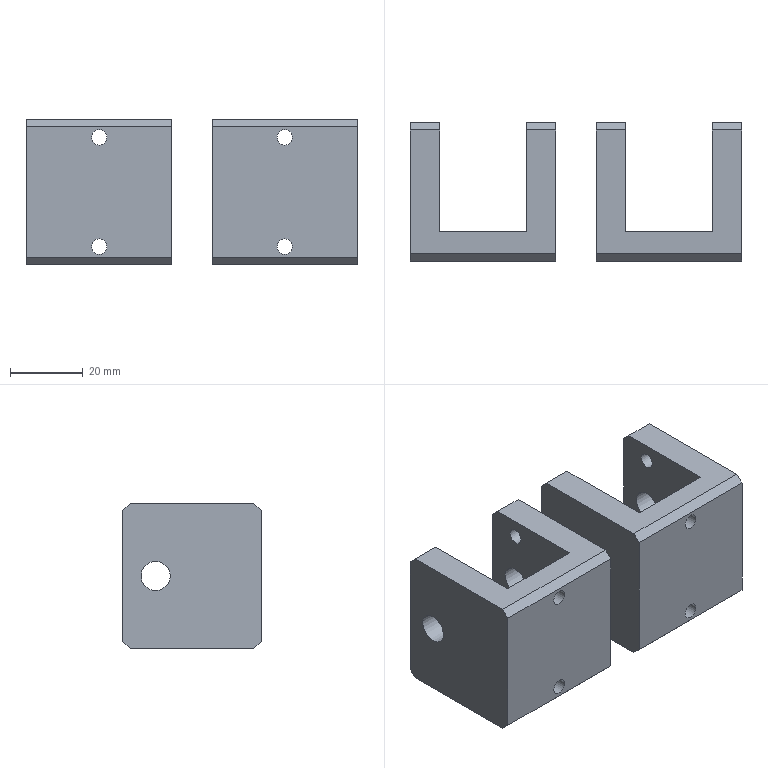Part | 2 solids | 52 faces | box 91 x 38 x 40 mm | volume 60346 mm3 | plane 32 | cylinder 16 | cone 4 | commonest cylinder face diameters 4.2 x12 8 x4
STEP:
#1=CARTESIAN_POINT('',(31.,36.,20.));
#2=VERTEX_POINT('',#1);
#3=CARTESIAN_POINT('',(31.,38.,18.));
#4=VERTEX_POINT('',#3);
#5=CARTESIAN_POINT('',(31.,38.,18.));
#6=DIRECTION('',(0.,0.7071,-0.7071));
#7=VECTOR('',#6,1000.);
#8=LINE('',#5,#7);
#9=EDGE_CURVE('',#2,#4,#8,.T.);
#10=ORIENTED_EDGE('',*,*,#9,.F.);
#11=CARTESIAN_POINT('',(39.,36.,20.));
#12=VERTEX_POINT('',#11);
#13=CARTESIAN_POINT('',(31.,36.,20.));
#14=DIRECTION('',(-1.,0.,0.));
#15=VECTOR('',#14,1000.);
#16=LINE('',#13,#15);
#17=EDGE_CURVE('',#12,#2,#16,.T.);
#18=ORIENTED_EDGE('',*,*,#17,.F.);
#19=CARTESIAN_POINT('',(39.,38.,18.));
#20=VERTEX_POINT('',#19);
#21=CARTESIAN_POINT('',(39.,38.,18.));
#22=DIRECTION('',(0.,-0.7071,0.7071));
#23=VECTOR('',#22,1000.);
#24=LINE('',#21,#23);
#25=EDGE_CURVE('',#20,#12,#24,.T.);
#26=ORIENTED_EDGE('',*,*,#25,.F.);
#27=CARTESIAN_POINT('',(39.,38.,18.));
#28=DIRECTION('',(1.,0.,0.));
#29=VECTOR('',#28,1000.);
#30=LINE('',#27,#29);
#31=EDGE_CURVE('',#4,#20,#30,.T.);
#32=ORIENTED_EDGE('',*,*,#31,.F.);
#33=EDGE_LOOP('',(#10,#18,#26,#32));
#34=FACE_BOUND('',#33,.T.);
#35=CARTESIAN_POINT('',(51.,38.,18.));
#36=DIRECTION('',(0.,0.7071,0.7071));
#37=DIRECTION('',(-1.,0.,0.));
#38=AXIS2_PLACEMENT_3D('',#35,#36,#37);
#39=PLANE('',#38);
#40=ADVANCED_FACE('',(#34),#39,.T.);
#41=CARTESIAN_POINT('',(39.,36.,-20.));
#42=VERTEX_POINT('',#41);
#43=CARTESIAN_POINT('',(39.,38.,-18.));
#44=VERTEX_POINT('',#43);
#45=CARTESIAN_POINT('',(39.,38.,-18.));
#46=DIRECTION('',(0.,0.7071,0.7071));
#47=VECTOR('',#46,1000.);
#48=LINE('',#45,#47);
#49=EDGE_CURVE('',#42,#44,#48,.T.);
#50=ORIENTED_EDGE('',*,*,#49,.F.);
#51=CARTESIAN_POINT('',(31.,36.,-20.));
#52=VERTEX_POINT('',#51);
#53=CARTESIAN_POINT('',(39.,36.,-20.));
#54=DIRECTION('',(1.,0.,0.));
#55=VECTOR('',#54,1000.);
#56=LINE('',#53,#55);
#57=EDGE_CURVE('',#52,#42,#56,.T.);
#58=ORIENTED_EDGE('',*,*,#57,.F.);
#59=CARTESIAN_POINT('',(31.,38.,-18.));
#60=VERTEX_POINT('',#59);
#61=CARTESIAN_POINT('',(31.,38.,-18.));
#62=DIRECTION('',(0.,-0.7071,-0.7071));
#63=VECTOR('',#62,1000.);
#64=LINE('',#61,#63);
#65=EDGE_CURVE('',#60,#52,#64,.T.);
#66=ORIENTED_EDGE('',*,*,#65,.F.);
#67=CARTESIAN_POINT('',(31.,38.,-18.));
#68=DIRECTION('',(-1.,0.,0.));
#69=VECTOR('',#68,1000.);
#70=LINE('',#67,#69);
#71=EDGE_CURVE('',#44,#60,#70,.T.);
#72=ORIENTED_EDGE('',*,*,#71,.F.);
#73=EDGE_LOOP('',(#50,#58,#66,#72));
#74=FACE_BOUND('',#73,.T.);
#75=CARTESIAN_POINT('',(51.,38.,-18.));
#76=DIRECTION('',(0.,0.7071,-0.7071));
#77=DIRECTION('',(1.,0.,0.));
#78=AXIS2_PLACEMENT_3D('',#75,#76,#77);
#79=PLANE('',#78);
#80=ADVANCED_FACE('',(#74),#79,.T.);
#81=CARTESIAN_POINT('',(71.,36.,-20.));
#82=VERTEX_POINT('',#81);
#83=CARTESIAN_POINT('',(71.,38.,-18.));
#84=VERTEX_POINT('',#83);
#85=CARTESIAN_POINT('',(71.,38.,-18.));
#86=DIRECTION('',(0.,0.7071,0.7071));
#87=VECTOR('',#86,1000.);
#88=LINE('',#85,#87);
#89=EDGE_CURVE('',#82,#84,#88,.T.);
#90=ORIENTED_EDGE('',*,*,#89,.F.);
#91=CARTESIAN_POINT('',(63.,36.,-20.));
#92=VERTEX_POINT('',#91);
#93=CARTESIAN_POINT('',(71.,36.,-20.));
#94=DIRECTION('',(1.,0.,0.));
#95=VECTOR('',#94,1000.);
#96=LINE('',#93,#95);
#97=EDGE_CURVE('',#92,#82,#96,.T.);
#98=ORIENTED_EDGE('',*,*,#97,.F.);
#99=CARTESIAN_POINT('',(63.,38.,-18.));
#100=VERTEX_POINT('',#99);
#101=CARTESIAN_POINT('',(63.,38.,-18.));
#102=DIRECTION('',(0.,-0.7071,-0.7071));
#103=VECTOR('',#102,1000.);
#104=LINE('',#101,#103);
#105=EDGE_CURVE('',#100,#92,#104,.T.);
#106=ORIENTED_EDGE('',*,*,#105,.F.);
#107=CARTESIAN_POINT('',(63.,38.,-18.));
#108=DIRECTION('',(-1.,0.,0.));
#109=VECTOR('',#108,1000.);
#110=LINE('',#107,#109);
#111=EDGE_CURVE('',#84,#100,#110,.T.);
#112=ORIENTED_EDGE('',*,*,#111,.F.);
#113=EDGE_LOOP('',(#90,#98,#106,#112));
#114=FACE_BOUND('',#113,.T.);
#115=CARTESIAN_POINT('',(51.,38.,-18.));
#116=DIRECTION('',(0.,0.7071,-0.7071));
#117=DIRECTION('',(1.,0.,0.));
#118=AXIS2_PLACEMENT_3D('',#115,#116,#117);
#119=PLANE('',#118);
#120=ADVANCED_FACE('',(#114),#119,.T.);
#121=CARTESIAN_POINT('',(63.,36.,20.));
#122=VERTEX_POINT('',#121);
#123=CARTESIAN_POINT('',(63.,38.,18.));
#124=VERTEX_POINT('',#123);
#125=CARTESIAN_POINT('',(63.,38.,18.));
#126=DIRECTION('',(0.,0.7071,-0.7071));
#127=VECTOR('',#126,1000.);
#128=LINE('',#125,#127);
#129=EDGE_CURVE('',#122,#124,#128,.T.);
#130=ORIENTED_EDGE('',*,*,#129,.F.);
#131=CARTESIAN_POINT('',(71.,36.,20.));
#132=VERTEX_POINT('',#131);
#133=CARTESIAN_POINT('',(63.,36.,20.));
#134=DIRECTION('',(-1.,0.,0.));
#135=VECTOR('',#134,1000.);
#136=LINE('',#133,#135);
#137=EDGE_CURVE('',#132,#122,#136,.T.);
#138=ORIENTED_EDGE('',*,*,#137,.F.);
#139=CARTESIAN_POINT('',(71.,38.,18.));
#140=VERTEX_POINT('',#139);
#141=CARTESIAN_POINT('',(71.,38.,18.));
#142=DIRECTION('',(0.,-0.7071,0.7071));
#143=VECTOR('',#142,1000.);
#144=LINE('',#141,#143);
#145=EDGE_CURVE('',#140,#132,#144,.T.);
#146=ORIENTED_EDGE('',*,*,#145,.F.);
#147=CARTESIAN_POINT('',(71.,38.,18.));
#148=DIRECTION('',(1.,0.,0.));
#149=VECTOR('',#148,1000.);
#150=LINE('',#147,#149);
#151=EDGE_CURVE('',#124,#140,#150,.T.);
#152=ORIENTED_EDGE('',*,*,#151,.F.);
#153=EDGE_LOOP('',(#130,#138,#146,#152));
#154=FACE_BOUND('',#153,.T.);
#155=CARTESIAN_POINT('',(51.,38.,18.));
#156=DIRECTION('',(0.,0.7071,0.7071));
#157=DIRECTION('',(-1.,0.,0.));
#158=AXIS2_PLACEMENT_3D('',#155,#156,#157);
#159=PLANE('',#158);
#160=ADVANCED_FACE('',(#154),#159,.T.);
#161=CARTESIAN_POINT('',(31.,0.,18.));
#162=VERTEX_POINT('',#161);
#163=CARTESIAN_POINT('',(31.,2.,20.));
#164=VERTEX_POINT('',#163);
#165=CARTESIAN_POINT('',(31.,2.,20.));
#166=DIRECTION('',(0.,0.7071,0.7071));
#167=VECTOR('',#166,1000.);
#168=LINE('',#165,#167);
#169=EDGE_CURVE('',#162,#164,#168,.T.);
#170=ORIENTED_EDGE('',*,*,#169,.F.);
#171=CARTESIAN_POINT('',(71.,0.,18.));
#172=VERTEX_POINT('',#171);
#173=CARTESIAN_POINT('',(51.,0.,18.));
#174=DIRECTION('',(-1.,0.,0.));
#175=VECTOR('',#174,1000.);
#176=LINE('',#173,#175);
#177=EDGE_CURVE('',#172,#162,#176,.T.);
#178=ORIENTED_EDGE('',*,*,#177,.F.);
#179=CARTESIAN_POINT('',(71.,2.,20.));
#180=VERTEX_POINT('',#179);
#181=CARTESIAN_POINT('',(71.,2.,20.));
#182=DIRECTION('',(0.,-0.7071,-0.7071));
#183=VECTOR('',#182,1000.);
#184=LINE('',#181,#183);
#185=EDGE_CURVE('',#180,#172,#184,.T.);
#186=ORIENTED_EDGE('',*,*,#185,.F.);
#187=CARTESIAN_POINT('',(31.,2.,20.));
#188=DIRECTION('',(1.,0.,0.));
#189=VECTOR('',#188,1000.);
#190=LINE('',#187,#189);
#191=EDGE_CURVE('',#164,#180,#190,.T.);
#192=ORIENTED_EDGE('',*,*,#191,.F.);
#193=EDGE_LOOP('',(#170,#178,#186,#192));
#194=FACE_BOUND('',#193,.T.);
#195=CARTESIAN_POINT('',(31.,2.,20.));
#196=DIRECTION('',(0.,0.7071,-0.7071));
#197=DIRECTION('',(1.,0.,0.));
#198=AXIS2_PLACEMENT_3D('',#195,#196,#197);
#199=PLANE('',#198);
#200=ADVANCED_FACE('',(#194),#199,.F.);
#201=CARTESIAN_POINT('',(71.,0.,-18.));
#202=VERTEX_POINT('',#201);
#203=CARTESIAN_POINT('',(71.,2.,-20.));
#204=VERTEX_POINT('',#203);
#205=CARTESIAN_POINT('',(71.,2.,-20.));
#206=DIRECTION('',(0.,0.7071,-0.7071));
#207=VECTOR('',#206,1000.);
#208=LINE('',#205,#207);
#209=EDGE_CURVE('',#202,#204,#208,.T.);
#210=ORIENTED_EDGE('',*,*,#209,.F.);
#211=CARTESIAN_POINT('',(31.,0.,-18.));
#212=VERTEX_POINT('',#211);
#213=CARTESIAN_POINT('',(51.,0.,-18.));
#214=DIRECTION('',(1.,0.,0.));
#215=VECTOR('',#214,1000.);
#216=LINE('',#213,#215);
#217=EDGE_CURVE('',#212,#202,#216,.T.);
#218=ORIENTED_EDGE('',*,*,#217,.F.);
#219=CARTESIAN_POINT('',(31.,2.,-20.));
#220=VERTEX_POINT('',#219);
#221=CARTESIAN_POINT('',(31.,2.,-20.));
#222=DIRECTION('',(0.,-0.7071,0.7071));
#223=VECTOR('',#222,1000.);
#224=LINE('',#221,#223);
#225=EDGE_CURVE('',#220,#212,#224,.T.);
#226=ORIENTED_EDGE('',*,*,#225,.F.);
#227=CARTESIAN_POINT('',(31.,2.,-20.));
#228=DIRECTION('',(-1.,0.,0.));
#229=VECTOR('',#228,1000.);
#230=LINE('',#227,#229);
#231=EDGE_CURVE('',#204,#220,#230,.T.);
#232=ORIENTED_EDGE('',*,*,#231,.F.);
#233=EDGE_LOOP('',(#210,#218,#226,#232));
#234=FACE_BOUND('',#233,.T.);
#235=CARTESIAN_POINT('',(31.,2.,-20.));
#236=DIRECTION('',(0.,0.7071,0.7071));
#237=DIRECTION('',(-1.,0.,0.));
#238=AXIS2_PLACEMENT_3D('',#235,#236,#237);
#239=PLANE('',#238);
#240=ADVANCED_FACE('',(#234),#239,.F.);
#241=CARTESIAN_POINT('',(63.,8.,20.));
#242=VERTEX_POINT('',#241);
#243=CARTESIAN_POINT('',(63.,8.,-20.));
#244=VERTEX_POINT('',#243);
#245=CARTESIAN_POINT('',(63.,8.,20.));
#246=DIRECTION('',(0.,0.,-1.));
#247=VECTOR('',#246,1000.);
#248=LINE('',#245,#247);
#249=EDGE_CURVE('',#242,#244,#248,.T.);
#250=ORIENTED_EDGE('',*,*,#249,.T.);
#251=CARTESIAN_POINT('',(39.,8.,-20.));
#252=VERTEX_POINT('',#251);
#253=CARTESIAN_POINT('',(39.,8.,-20.));
#254=DIRECTION('',(-1.,0.,0.));
#255=VECTOR('',#254,1000.);
#256=LINE('',#253,#255);
#257=EDGE_CURVE('',#244,#252,#256,.T.);
#258=ORIENTED_EDGE('',*,*,#257,.T.);
#259=CARTESIAN_POINT('',(39.,8.,20.));
#260=VERTEX_POINT('',#259);
#261=CARTESIAN_POINT('',(39.,8.,20.));
#262=DIRECTION('',(0.,0.,1.));
#263=VECTOR('',#262,1000.);
#264=LINE('',#261,#263);
#265=EDGE_CURVE('',#252,#260,#264,.T.);
#266=ORIENTED_EDGE('',*,*,#265,.T.);
#267=CARTESIAN_POINT('',(39.,8.,20.));
#268=DIRECTION('',(1.,0.,0.));
#269=VECTOR('',#268,1000.);
#270=LINE('',#267,#269);
#271=EDGE_CURVE('',#260,#242,#270,.T.);
#272=ORIENTED_EDGE('',*,*,#271,.T.);
#273=EDGE_LOOP('',(#250,#258,#266,#272));
#274=FACE_BOUND('',#273,.T.);
#275=CARTESIAN_POINT('',(51.,8.,-17.1));
#276=VERTEX_POINT('',#275);
#277=CARTESIAN_POINT('',(51.,8.,-15.));
#278=DIRECTION('',(0.,-1.,0.));
#279=DIRECTION('',(0.,0.,-1.));
#280=AXIS2_PLACEMENT_3D('',#277,#278,#279);
#281=CIRCLE('',#280,2.1);
#282=EDGE_CURVE('',#276,#276,#281,.T.);
#283=ORIENTED_EDGE('',*,*,#282,.T.);
#284=EDGE_LOOP('',(#283));
#285=FACE_BOUND('',#284,.T.);
#286=CARTESIAN_POINT('',(51.,8.,12.9));
#287=VERTEX_POINT('',#286);
#288=CARTESIAN_POINT('',(51.,8.,15.));
#289=DIRECTION('',(0.,-1.,0.));
#290=DIRECTION('',(0.,0.,-1.));
#291=AXIS2_PLACEMENT_3D('',#288,#289,#290);
#292=CIRCLE('',#291,2.1);
#293=EDGE_CURVE('',#287,#287,#292,.T.);
#294=ORIENTED_EDGE('',*,*,#293,.T.);
#295=EDGE_LOOP('',(#294));
#296=FACE_BOUND('',#295,.T.);
#297=CARTESIAN_POINT('',(51.,8.,0.));
#298=DIRECTION('',(0.,-1.,0.));
#299=DIRECTION('',(0.,0.,-1.));
#300=AXIS2_PLACEMENT_3D('',#297,#298,#299);
#301=PLANE('',#300);
#302=ADVANCED_FACE('',(#274,#285,#296),#301,.F.);
#303=CARTESIAN_POINT('',(39.,8.,-20.));
#304=DIRECTION('',(0.,1.,0.));
#305=VECTOR('',#304,1000.);
#306=LINE('',#303,#305);
#307=EDGE_CURVE('',#252,#42,#306,.T.);
#308=ORIENTED_EDGE('',*,*,#307,.T.);
#309=ORIENTED_EDGE('',*,*,#49,.T.);
#310=CARTESIAN_POINT('',(39.,38.,20.));
#311=DIRECTION('',(0.,0.,1.));
#312=VECTOR('',#311,1000.);
#313=LINE('',#310,#312);
#314=EDGE_CURVE('',#44,#20,#313,.T.);
#315=ORIENTED_EDGE('',*,*,#314,.T.);
#316=ORIENTED_EDGE('',*,*,#25,.T.);
#317=CARTESIAN_POINT('',(39.,8.,20.));
#318=DIRECTION('',(0.,1.,0.));
#319=VECTOR('',#318,1000.);
#320=LINE('',#317,#319);
#321=EDGE_CURVE('',#260,#12,#320,.T.);
#322=ORIENTED_EDGE('',*,*,#321,.F.);
#323=ORIENTED_EDGE('',*,*,#265,.F.);
#324=EDGE_LOOP('',(#308,#309,#315,#316,#322,#323));
#325=FACE_BOUND('',#324,.T.);
#326=CARTESIAN_POINT('',(39.,29.,4.));
#327=VERTEX_POINT('',#326);
#328=CARTESIAN_POINT('',(39.,29.,0.));
#329=DIRECTION('',(-1.,0.,0.));
#330=DIRECTION('',(0.,0.,1.));
#331=AXIS2_PLACEMENT_3D('',#328,#329,#330);
#332=CIRCLE('',#331,4.);
#333=EDGE_CURVE('',#327,#327,#332,.T.);
#334=ORIENTED_EDGE('',*,*,#333,.T.);
#335=EDGE_LOOP('',(#334));
#336=FACE_BOUND('',#335,.T.);
#337=CARTESIAN_POINT('',(39.,8.,20.));
#338=DIRECTION('',(-1.,0.,0.));
#339=DIRECTION('',(0.,0.,1.));
#340=AXIS2_PLACEMENT_3D('',#337,#338,#339);
#341=PLANE('',#340);
#342=ADVANCED_FACE('',(#325,#336),#341,.F.);
#343=CARTESIAN_POINT('',(63.,8.,20.));
#344=DIRECTION('',(0.,1.,0.));
#345=VECTOR('',#344,1000.);
#346=LINE('',#343,#345);
#347=EDGE_CURVE('',#242,#122,#346,.T.);
#348=ORIENTED_EDGE('',*,*,#347,.T.);
#349=ORIENTED_EDGE('',*,*,#129,.T.);
#350=CARTESIAN_POINT('',(63.,38.,20.));
#351=DIRECTION('',(0.,0.,-1.));
#352=VECTOR('',#351,1000.);
#353=LINE('',#350,#352);
#354=EDGE_CURVE('',#124,#100,#353,.T.);
#355=ORIENTED_EDGE('',*,*,#354,.T.);
#356=ORIENTED_EDGE('',*,*,#105,.T.);
#357=CARTESIAN_POINT('',(63.,8.,-20.));
#358=DIRECTION('',(0.,1.,0.));
#359=VECTOR('',#358,1000.);
#360=LINE('',#357,#359);
#361=EDGE_CURVE('',#244,#92,#360,.T.);
#362=ORIENTED_EDGE('',*,*,#361,.F.);
#363=ORIENTED_EDGE('',*,*,#249,.F.);
#364=EDGE_LOOP('',(#348,#349,#355,#356,#362,#363));
#365=FACE_BOUND('',#364,.T.);
#366=CARTESIAN_POINT('',(63.,29.,-4.));
#367=VERTEX_POINT('',#366);
#368=CARTESIAN_POINT('',(63.,29.,0.));
#369=DIRECTION('',(1.,0.,0.));
#370=DIRECTION('',(0.,0.,-1.));
#371=AXIS2_PLACEMENT_3D('',#368,#369,#370);
#372=CIRCLE('',#371,4.);
#373=EDGE_CURVE('',#367,#367,#372,.T.);
#374=ORIENTED_EDGE('',*,*,#373,.T.);
#375=EDGE_LOOP('',(#374));
#376=FACE_BOUND('',#375,.T.);
#377=CARTESIAN_POINT('',(63.,29.,12.9));
#378=VERTEX_POINT('',#377);
#379=CARTESIAN_POINT('',(63.,29.,15.));
#380=DIRECTION('',(1.,0.,0.));
#381=DIRECTION('',(0.,0.,-1.));
#382=AXIS2_PLACEMENT_3D('',#379,#380,#381);
#383=CIRCLE('',#382,2.1);
#384=EDGE_CURVE('',#378,#378,#383,.T.);
#385=ORIENTED_EDGE('',*,*,#384,.T.);
#386=EDGE_LOOP('',(#385));
#387=FACE_BOUND('',#386,.T.);
#388=CARTESIAN_POINT('',(63.,29.,-17.1));
#389=VERTEX_POINT('',#388);
#390=CARTESIAN_POINT('',(63.,29.,-15.));
#391=DIRECTION('',(1.,0.,0.));
#392=DIRECTION('',(0.,0.,-1.));
#393=AXIS2_PLACEMENT_3D('',#390,#391,#392);
#394=CIRCLE('',#393,2.1);
#395=EDGE_CURVE('',#389,#389,#394,.T.);
#396=ORIENTED_EDGE('',*,*,#395,.T.);
#397=EDGE_LOOP('',(#396));
#398=FACE_BOUND('',#397,.T.);
#399=CARTESIAN_POINT('',(63.,8.,20.));
#400=DIRECTION('',(1.,0.,0.));
#401=DIRECTION('',(0.,0.,-1.));
#402=AXIS2_PLACEMENT_3D('',#399,#400,#401);
#403=PLANE('',#402);
#404=ADVANCED_FACE('',(#365,#376,#387,#398),#403,.F.);
#405=CARTESIAN_POINT('',(31.,0.,-20.));
#406=DIRECTION('',(0.,0.,1.));
#407=VECTOR('',#406,1000.);
#408=LINE('',#405,#407);
#409=EDGE_CURVE('',#212,#162,#408,.T.);
#410=ORIENTED_EDGE('',*,*,#409,.F.);
#411=ORIENTED_EDGE('',*,*,#217,.T.);
#412=CARTESIAN_POINT('',(71.,0.,-20.));
#413=DIRECTION('',(0.,0.,-1.));
#414=VECTOR('',#413,1000.);
#415=LINE('',#412,#414);
#416=EDGE_CURVE('',#172,#202,#415,.T.);
#417=ORIENTED_EDGE('',*,*,#416,.F.);
#418=ORIENTED_EDGE('',*,*,#177,.T.);
#419=EDGE_LOOP('',(#410,#411,#417,#418));
#420=FACE_BOUND('',#419,.T.);
#421=CARTESIAN_POINT('',(51.,0.,-17.1));
#422=VERTEX_POINT('',#421);
#423=CARTESIAN_POINT('',(51.,0.,-15.));
#424=DIRECTION('',(0.,-1.,0.));
#425=DIRECTION('',(0.,0.,-1.));
#426=AXIS2_PLACEMENT_3D('',#423,#424,#425);
#427=CIRCLE('',#426,2.1);
#428=EDGE_CURVE('',#422,#422,#427,.T.);
#429=ORIENTED_EDGE('',*,*,#428,.F.);
#430=EDGE_LOOP('',(#429));
#431=FACE_BOUND('',#430,.T.);
#432=CARTESIAN_POINT('',(51.,0.,12.9));
#433=VERTEX_POINT('',#432);
#434=CARTESIAN_POINT('',(51.,0.,15.));
#435=DIRECTION('',(0.,-1.,0.));
#436=DIRECTION('',(0.,0.,-1.));
#437=AXIS2_PLACEMENT_3D('',#434,#435,#436);
#438=CIRCLE('',#437,2.1);
#439=EDGE_CURVE('',#433,#433,#438,.T.);
#440=ORIENTED_EDGE('',*,*,#439,.F.);
#441=EDGE_LOOP('',(#440));
#442=FACE_BOUND('',#441,.T.);
#443=CARTESIAN_POINT('',(51.,0.,0.));
#444=DIRECTION('',(0.,1.,0.));
#445=DIRECTION('',(0.,0.,1.));
#446=AXIS2_PLACEMENT_3D('',#443,#444,#445);
#447=PLANE('',#446);
#448=ADVANCED_FACE('',(#420,#431,#442),#447,.F.);
#449=ORIENTED_EDGE('',*,*,#314,.F.);
#450=ORIENTED_EDGE('',*,*,#71,.T.);
#451=CARTESIAN_POINT('',(31.,38.,-20.));
#452=DIRECTION('',(0.,0.,1.));
#453=VECTOR('',#452,1000.);
#454=LINE('',#451,#453);
#455=EDGE_CURVE('',#60,#4,#454,.T.);
#456=ORIENTED_EDGE('',*,*,#455,.T.);
#457=ORIENTED_EDGE('',*,*,#31,.T.);
#458=EDGE_LOOP('',(#449,#450,#456,#457));
#459=FACE_BOUND('',#458,.T.);
#460=CARTESIAN_POINT('',(51.,38.,0.));
#461=DIRECTION('',(0.,1.,0.));
#462=DIRECTION('',(0.,0.,1.));
#463=AXIS2_PLACEMENT_3D('',#460,#461,#462);
#464=PLANE('',#463);
#465=ADVANCED_FACE('',(#459),#464,.T.);
#466=CARTESIAN_POINT('',(31.,38.,20.));
#467=DIRECTION('',(0.,-1.,0.));
#468=VECTOR('',#467,1000.);
#469=LINE('',#466,#468);
#470=EDGE_CURVE('',#2,#164,#469,.T.);
#471=ORIENTED_EDGE('',*,*,#470,.T.);
#472=ORIENTED_EDGE('',*,*,#191,.T.);
#473=CARTESIAN_POINT('',(71.,38.,20.));
#474=DIRECTION('',(0.,-1.,0.));
#475=VECTOR('',#474,1000.);
#476=LINE('',#473,#475);
#477=EDGE_CURVE('',#132,#180,#476,.T.);
#478=ORIENTED_EDGE('',*,*,#477,.F.);
#479=ORIENTED_EDGE('',*,*,#137,.T.);
#480=ORIENTED_EDGE('',*,*,#347,.F.);
#481=ORIENTED_EDGE('',*,*,#271,.F.);
#482=ORIENTED_EDGE('',*,*,#321,.T.);
#483=ORIENTED_EDGE('',*,*,#17,.T.);
#484=EDGE_LOOP('',(#471,#472,#478,#479,#480,#481,#482,#483));
#485=FACE_BOUND('',#484,.T.);
#486=CARTESIAN_POINT('',(31.,38.,20.));
#487=DIRECTION('',(0.,0.,-1.));
#488=DIRECTION('',(-1.,0.,0.));
#489=AXIS2_PLACEMENT_3D('',#486,#487,#488);
#490=PLANE('',#489);
#491=ADVANCED_FACE('',(#485),#490,.F.);
#492=CARTESIAN_POINT('',(31.,38.,-20.));
#493=DIRECTION('',(0.,-1.,0.));
#494=VECTOR('',#493,1000.);
#495=LINE('',#492,#494);
#496=EDGE_CURVE('',#52,#220,#495,.T.);
#497=ORIENTED_EDGE('',*,*,#496,.T.);
#498=ORIENTED_EDGE('',*,*,#225,.T.);
#499=ORIENTED_EDGE('',*,*,#409,.T.);
#500=ORIENTED_EDGE('',*,*,#169,.T.);
#501=ORIENTED_EDGE('',*,*,#470,.F.);
#502=ORIENTED_EDGE('',*,*,#9,.T.);
#503=ORIENTED_EDGE('',*,*,#455,.F.);
#504=ORIENTED_EDGE('',*,*,#65,.T.);
#505=EDGE_LOOP('',(#497,#498,#499,#500,#501,#502,#503,#504));
#506=FACE_BOUND('',#505,.T.);
#507=CARTESIAN_POINT('',(31.,29.,-4.));
#508=VERTEX_POINT('',#507);
#509=CARTESIAN_POINT('',(31.,29.,0.));
#510=DIRECTION('',(1.,0.,0.));
#511=DIRECTION('',(0.,0.,-1.));
#512=AXIS2_PLACEMENT_3D('',#509,#510,#511);
#513=CIRCLE('',#512,4.);
#514=EDGE_CURVE('',#508,#508,#513,.T.);
#515=ORIENTED_EDGE('',*,*,#514,.T.);
#516=EDGE_LOOP('',(#515));
#517=FACE_BOUND('',#516,.T.);
#518=CARTESIAN_POINT('',(31.,38.,-20.));
#519=DIRECTION('',(1.,0.,0.));
#520=DIRECTION('',(0.,0.,-1.));
#521=AXIS2_PLACEMENT_3D('',#518,#519,#520);
#522=PLANE('',#521);
#523=ADVANCED_FACE('',(#506,#517),#522,.F.);
#524=CARTESIAN_POINT('',(71.,38.,-20.));
#525=DIRECTION('',(0.,-1.,0.));
#526=VECTOR('',#525,1000.);
#527=LINE('',#524,#526);
#528=EDGE_CURVE('',#82,#204,#527,.T.);
#529=ORIENTED_EDGE('',*,*,#528,.T.);
#530=ORIENTED_EDGE('',*,*,#231,.T.);
#531=ORIENTED_EDGE('',*,*,#496,.F.);
#532=ORIENTED_EDGE('',*,*,#57,.T.);
#533=ORIENTED_EDGE('',*,*,#307,.F.);
#534=ORIENTED_EDGE('',*,*,#257,.F.);
#535=ORIENTED_EDGE('',*,*,#361,.T.);
#536=ORIENTED_EDGE('',*,*,#97,.T.);
#537=EDGE_LOOP('',(#529,#530,#531,#532,#533,#534,#535,#536));
#538=FACE_BOUND('',#537,.T.);
#539=CARTESIAN_POINT('',(31.,38.,-20.));
#540=DIRECTION('',(0.,0.,1.));
#541=DIRECTION('',(1.,0.,0.));
#542=AXIS2_PLACEMENT_3D('',#539,#540,#541);
#543=PLANE('',#542);
#544=ADVANCED_FACE('',(#538),#543,.F.);
#545=ORIENTED_EDGE('',*,*,#416,.T.);
#546=ORIENTED_EDGE('',*,*,#209,.T.);
#547=ORIENTED_EDGE('',*,*,#528,.F.);
#548=ORIENTED_EDGE('',*,*,#89,.T.);
#549=CARTESIAN_POINT('',(71.,38.,-20.));
#550=DIRECTION('',(0.,0.,-1.));
#551=VECTOR('',#550,1000.);
#552=LINE('',#549,#551);
#553=EDGE_CURVE('',#140,#84,#552,.T.);
#554=ORIENTED_EDGE('',*,*,#553,.F.);
#555=ORIENTED_EDGE('',*,*,#145,.T.);
#556=ORIENTED_EDGE('',*,*,#477,.T.);
#557=ORIENTED_EDGE('',*,*,#185,.T.);
#558=EDGE_LOOP('',(#545,#546,#547,#548,#554,#555,#556,#557));
#559=FACE_BOUND('',#558,.T.);
#560=CARTESIAN_POINT('',(71.,29.,-4.));
#561=VERTEX_POINT('',#560);
#562=CARTESIAN_POINT('',(71.,29.,0.));
#563=DIRECTION('',(1.,0.,0.));
#564=DIRECTION('',(0.,0.,-1.));
#565=AXIS2_PLACEMENT_3D('',#562,#563,#564);
#566=CIRCLE('',#565,4.);
#567=EDGE_CURVE('',#561,#561,#566,.T.);
#568=ORIENTED_EDGE('',*,*,#567,.F.);
#569=EDGE_LOOP('',(#568));
#570=FACE_BOUND('',#569,.T.);
#571=CARTESIAN_POINT('',(71.,4.,12.9));
#572=VERTEX_POINT('',#571);
#573=CARTESIAN_POINT('',(71.,4.,15.));
#574=DIRECTION('',(1.,0.,0.));
#575=DIRECTION('',(0.,0.,-1.));
#576=AXIS2_PLACEMENT_3D('',#573,#574,#575);
#577=CIRCLE('',#576,2.1);
#578=EDGE_CURVE('',#572,#572,#577,.T.);
#579=ORIENTED_EDGE('',*,*,#578,.F.);
#580=EDGE_LOOP('',(#579));
#581=FACE_BOUND('',#580,.T.);
#582=CARTESIAN_POINT('',(71.,29.,12.9));
#583=VERTEX_POINT('',#582);
#584=CARTESIAN_POINT('',(71.,29.,15.));
#585=DIRECTION('',(1.,0.,0.));
#586=DIRECTION('',(0.,0.,-1.));
#587=AXIS2_PLACEMENT_3D('',#584,#585,#586);
#588=CIRCLE('',#587,2.1);
#589=EDGE_CURVE('',#583,#583,#588,.T.);
#590=ORIENTED_EDGE('',*,*,#589,.F.);
#591=EDGE_LOOP('',(#590));
#592=FACE_BOUND('',#591,.T.);
#593=CARTESIAN_POINT('',(71.,4.,-17.1));
#594=VERTEX_POINT('',#593);
#595=CARTESIAN_POINT('',(71.,4.,-15.));
#596=DIRECTION('',(1.,0.,0.));
#597=DIRECTION('',(0.,0.,-1.));
#598=AXIS2_PLACEMENT_3D('',#595,#596,#597);
#599=CIRCLE('',#598,2.1);
#600=EDGE_CURVE('',#594,#594,#599,.T.);
#601=ORIENTED_EDGE('',*,*,#600,.F.);
#602=EDGE_LOOP('',(#601));
#603=FACE_BOUND('',#602,.T.);
#604=CARTESIAN_POINT('',(71.,29.,-17.1));
#605=VERTEX_POINT('',#604);
#606=CARTESIAN_POINT('',(71.,29.,-15.));
#607=DIRECTION('',(1.,0.,0.));
#608=DIRECTION('',(0.,0.,-1.));
#609=AXIS2_PLACEMENT_3D('',#606,#607,#608);
#610=CIRCLE('',#609,2.1);
#611=EDGE_CURVE('',#605,#605,#610,.T.);
#612=ORIENTED_EDGE('',*,*,#611,.F.);
#613=EDGE_LOOP('',(#612));
#614=FACE_BOUND('',#613,.T.);
#615=CARTESIAN_POINT('',(71.,38.,-20.));
#616=DIRECTION('',(-1.,0.,0.));
#617=DIRECTION('',(0.,0.,1.));
#618=AXIS2_PLACEMENT_3D('',#615,#616,#617);
#619=PLANE('',#618);
#620=ADVANCED_FACE('',(#559,#570,#581,#592,#603,#614),#619,.F.);
#621=ORIENTED_EDGE('',*,*,#354,.F.);
#622=ORIENTED_EDGE('',*,*,#151,.T.);
#623=ORIENTED_EDGE('',*,*,#553,.T.);
#624=ORIENTED_EDGE('',*,*,#111,.T.);
#625=EDGE_LOOP('',(#621,#622,#623,#624));
#626=FACE_BOUND('',#625,.T.);
#627=CARTESIAN_POINT('',(51.,38.,0.));
#628=DIRECTION('',(0.,1.,0.));
#629=DIRECTION('',(0.,0.,1.));
#630=AXIS2_PLACEMENT_3D('',#627,#628,#629);
#631=PLANE('',#630);
#632=ADVANCED_FACE('',(#626),#631,.T.);
#633=ORIENTED_EDGE('',*,*,#333,.F.);
#634=EDGE_LOOP('',(#633));
#635=FACE_BOUND('',#634,.T.);
#636=ORIENTED_EDGE('',*,*,#514,.F.);
#637=EDGE_LOOP('',(#636));
#638=FACE_BOUND('',#637,.T.);
#639=CARTESIAN_POINT('',(24.,29.,0.));
#640=DIRECTION('',(1.,0.,0.));
#641=DIRECTION('',(0.,0.,-1.));
#642=AXIS2_PLACEMENT_3D('',#639,#640,#641);
#643=CYLINDRICAL_SURFACE('',#642,4.);
#644=ADVANCED_FACE('',(#635,#638),#643,.F.);
#645=ORIENTED_EDGE('',*,*,#567,.T.);
#646=EDGE_LOOP('',(#645));
#647=FACE_BOUND('',#646,.T.);
#648=ORIENTED_EDGE('',*,*,#373,.F.);
#649=EDGE_LOOP('',(#648));
#650=FACE_BOUND('',#649,.T.);
#651=CARTESIAN_POINT('',(24.,29.,0.));
#652=DIRECTION('',(1.,0.,0.));
#653=DIRECTION('',(0.,0.,-1.));
#654=AXIS2_PLACEMENT_3D('',#651,#652,#653);
#655=CYLINDRICAL_SURFACE('',#654,4.);
#656=ADVANCED_FACE('',(#647,#650),#655,.F.);
#657=CARTESIAN_POINT('',(57.338,4.,15.));
#658=VERTEX_POINT('',#657);
#659=VERTEX_LOOP('',#658);
#660=FACE_BOUND('',#659,.T.);
#661=CARTESIAN_POINT('',(58.6,4.,12.9));
#662=VERTEX_POINT('',#661);
#663=CARTESIAN_POINT('',(58.6,4.,15.));
#664=DIRECTION('',(1.,0.,0.));
#665=DIRECTION('',(0.,0.,-1.));
#666=AXIS2_PLACEMENT_3D('',#663,#664,#665);
#667=CIRCLE('',#666,2.1);
#668=EDGE_CURVE('',#662,#662,#667,.T.);
#669=ORIENTED_EDGE('',*,*,#668,.T.);
#670=EDGE_LOOP('',(#669));
#671=FACE_BOUND('',#670,.T.);
#672=CARTESIAN_POINT('',(58.6,4.,15.));
#673=DIRECTION('',(1.,0.,0.));
#674=DIRECTION('',(0.,0.,-1.));
#675=AXIS2_PLACEMENT_3D('',#672,#673,#674);
#676=CONICAL_SURFACE('',#675,2.1,1.03);
#677=ADVANCED_FACE('',(#660,#671),#676,.F.);
#678=ORIENTED_EDGE('',*,*,#578,.T.);
#679=EDGE_LOOP('',(#678));
#680=FACE_BOUND('',#679,.T.);
#681=ORIENTED_EDGE('',*,*,#668,.F.);
#682=EDGE_LOOP('',(#681));
#683=FACE_BOUND('',#682,.T.);
#684=CARTESIAN_POINT('',(71.,4.,15.));
#685=DIRECTION('',(1.,0.,0.));
#686=DIRECTION('',(0.,0.,-1.));
#687=AXIS2_PLACEMENT_3D('',#684,#685,#686);
#688=CYLINDRICAL_SURFACE('',#687,2.1);
#689=ADVANCED_FACE('',(#680,#683),#688,.F.);
#690=ORIENTED_EDGE('',*,*,#589,.T.);
#691=EDGE_LOOP('',(#690));
#692=FACE_BOUND('',#691,.T.);
#693=ORIENTED_EDGE('',*,*,#384,.F.);
#694=EDGE_LOOP('',(#693));
#695=FACE_BOUND('',#694,.T.);
#696=CARTESIAN_POINT('',(71.,29.,15.));
#697=DIRECTION('',(1.,0.,0.));
#698=DIRECTION('',(0.,0.,-1.));
#699=AXIS2_PLACEMENT_3D('',#696,#697,#698);
#700=CYLINDRICAL_SURFACE('',#699,2.1);
#701=ADVANCED_FACE('',(#692,#695),#700,.F.);
#702=CARTESIAN_POINT('',(57.338,4.,-15.));
#703=VERTEX_POINT('',#702);
#704=VERTEX_LOOP('',#703);
#705=FACE_BOUND('',#704,.T.);
#706=CARTESIAN_POINT('',(58.6,4.,-17.1));
#707=VERTEX_POINT('',#706);
#708=CARTESIAN_POINT('',(58.6,4.,-15.));
#709=DIRECTION('',(1.,0.,0.));
#710=DIRECTION('',(0.,0.,-1.));
#711=AXIS2_PLACEMENT_3D('',#708,#709,#710);
#712=CIRCLE('',#711,2.1);
#713=EDGE_CURVE('',#707,#707,#712,.T.);
#714=ORIENTED_EDGE('',*,*,#713,.T.);
#715=EDGE_LOOP('',(#714));
#716=FACE_BOUND('',#715,.T.);
#717=CARTESIAN_POINT('',(58.6,4.,-15.));
#718=DIRECTION('',(1.,0.,0.));
#719=DIRECTION('',(0.,0.,-1.));
#720=AXIS2_PLACEMENT_3D('',#717,#718,#719);
#721=CONICAL_SURFACE('',#720,2.1,1.03);
#722=ADVANCED_FACE('',(#705,#716),#721,.F.);
#723=ORIENTED_EDGE('',*,*,#600,.T.);
#724=EDGE_LOOP('',(#723));
#725=FACE_BOUND('',#724,.T.);
#726=ORIENTED_EDGE('',*,*,#713,.F.);
#727=EDGE_LOOP('',(#726));
#728=FACE_BOUND('',#727,.T.);
#729=CARTESIAN_POINT('',(71.,4.,-15.));
#730=DIRECTION('',(1.,0.,0.));
#731=DIRECTION('',(0.,0.,-1.));
#732=AXIS2_PLACEMENT_3D('',#729,#730,#731);
#733=CYLINDRICAL_SURFACE('',#732,2.1);
#734=ADVANCED_FACE('',(#725,#728),#733,.F.);
#735=ORIENTED_EDGE('',*,*,#611,.T.);
#736=EDGE_LOOP('',(#735));
#737=FACE_BOUND('',#736,.T.);
#738=ORIENTED_EDGE('',*,*,#395,.F.);
#739=EDGE_LOOP('',(#738));
#740=FACE_BOUND('',#739,.T.);
#741=CARTESIAN_POINT('',(71.,29.,-15.));
#742=DIRECTION('',(1.,0.,0.));
#743=DIRECTION('',(0.,0.,-1.));
#744=AXIS2_PLACEMENT_3D('',#741,#742,#743);
#745=CYLINDRICAL_SURFACE('',#744,2.1);
#746=ADVANCED_FACE('',(#737,#740),#745,.F.);
#747=ORIENTED_EDGE('',*,*,#428,.T.);
#748=EDGE_LOOP('',(#747));
#749=FACE_BOUND('',#748,.T.);
#750=ORIENTED_EDGE('',*,*,#282,.F.);
#751=EDGE_LOOP('',(#750));
#752=FACE_BOUND('',#751,.T.);
#753=CARTESIAN_POINT('',(51.,0.,-15.));
#754=DIRECTION('',(0.,-1.,0.));
#755=DIRECTION('',(0.,0.,-1.));
#756=AXIS2_PLACEMENT_3D('',#753,#754,#755);
#757=CYLINDRICAL_SURFACE('',#756,2.1);
#758=ADVANCED_FACE('',(#749,#752),#757,.F.);
#759=ORIENTED_EDGE('',*,*,#439,.T.);
#760=EDGE_LOOP('',(#759));
#761=FACE_BOUND('',#760,.T.);
#762=ORIENTED_EDGE('',*,*,#293,.F.);
#763=EDGE_LOOP('',(#762));
#764=FACE_BOUND('',#763,.T.);
#765=CARTESIAN_POINT('',(51.,0.,15.));
#766=DIRECTION('',(0.,-1.,0.));
#767=DIRECTION('',(0.,0.,-1.));
#768=AXIS2_PLACEMENT_3D('',#765,#766,#767);
#769=CYLINDRICAL_SURFACE('',#768,2.1);
#770=ADVANCED_FACE('',(#761,#764),#769,.F.);
#771=CLOSED_SHELL('',(#40,#80,#120,#160,#200,#240,#302,#342,#404,#448,#465,#491,#523,#544,#620,#632,#644,#656,#677,#689,#701,#722,#734,#746,#758,#770));
#772=MANIFOLD_SOLID_BREP('',#771);
#773=CARTESIAN_POINT('',(-20.,36.,20.));
#774=VERTEX_POINT('',#773);
#775=CARTESIAN_POINT('',(-20.,38.,18.));
#776=VERTEX_POINT('',#775);
#777=CARTESIAN_POINT('',(-20.,38.,18.));
#778=DIRECTION('',(0.,0.7071,-0.7071));
#779=VECTOR('',#778,1000.);
#780=LINE('',#777,#779);
#781=EDGE_CURVE('',#774,#776,#780,.T.);
#782=ORIENTED_EDGE('',*,*,#781,.F.);
#783=CARTESIAN_POINT('',(-12.,36.,20.));
#784=VERTEX_POINT('',#783);
#785=CARTESIAN_POINT('',(-20.,36.,20.));
#786=DIRECTION('',(-1.,0.,0.));
#787=VECTOR('',#786,1000.);
#788=LINE('',#785,#787);
#789=EDGE_CURVE('',#784,#774,#788,.T.);
#790=ORIENTED_EDGE('',*,*,#789,.F.);
#791=CARTESIAN_POINT('',(-12.,38.,18.));
#792=VERTEX_POINT('',#791);
#793=CARTESIAN_POINT('',(-12.,38.,18.));
#794=DIRECTION('',(0.,-0.7071,0.7071));
#795=VECTOR('',#794,1000.);
#796=LINE('',#793,#795);
#797=EDGE_CURVE('',#792,#784,#796,.T.);
#798=ORIENTED_EDGE('',*,*,#797,.F.);
#799=CARTESIAN_POINT('',(-12.,38.,18.));
#800=DIRECTION('',(1.,0.,0.));
#801=VECTOR('',#800,1000.);
#802=LINE('',#799,#801);
#803=EDGE_CURVE('',#776,#792,#802,.T.);
#804=ORIENTED_EDGE('',*,*,#803,.F.);
#805=EDGE_LOOP('',(#782,#790,#798,#804));
#806=FACE_BOUND('',#805,.T.);
#807=CARTESIAN_POINT('',(0.,38.,18.));
#808=DIRECTION('',(0.,0.7071,0.7071));
#809=DIRECTION('',(-1.,0.,0.));
#810=AXIS2_PLACEMENT_3D('',#807,#808,#809);
#811=PLANE('',#810);
#812=ADVANCED_FACE('',(#806),#811,.T.);
#813=CARTESIAN_POINT('',(-12.,36.,-20.));
#814=VERTEX_POINT('',#813);
#815=CARTESIAN_POINT('',(-12.,38.,-18.));
#816=VERTEX_POINT('',#815);
#817=CARTESIAN_POINT('',(-12.,38.,-18.));
#818=DIRECTION('',(0.,0.7071,0.7071));
#819=VECTOR('',#818,1000.);
#820=LINE('',#817,#819);
#821=EDGE_CURVE('',#814,#816,#820,.T.);
#822=ORIENTED_EDGE('',*,*,#821,.F.);
#823=CARTESIAN_POINT('',(-20.,36.,-20.));
#824=VERTEX_POINT('',#823);
#825=CARTESIAN_POINT('',(-12.,36.,-20.));
#826=DIRECTION('',(1.,0.,0.));
#827=VECTOR('',#826,1000.);
#828=LINE('',#825,#827);
#829=EDGE_CURVE('',#824,#814,#828,.T.);
#830=ORIENTED_EDGE('',*,*,#829,.F.);
#831=CARTESIAN_POINT('',(-20.,38.,-18.));
#832=VERTEX_POINT('',#831);
#833=CARTESIAN_POINT('',(-20.,38.,-18.));
#834=DIRECTION('',(0.,-0.7071,-0.7071));
#835=VECTOR('',#834,1000.);
#836=LINE('',#833,#835);
#837=EDGE_CURVE('',#832,#824,#836,.T.);
#838=ORIENTED_EDGE('',*,*,#837,.F.);
#839=CARTESIAN_POINT('',(-20.,38.,-18.));
#840=DIRECTION('',(-1.,0.,0.));
#841=VECTOR('',#840,1000.);
#842=LINE('',#839,#841);
#843=EDGE_CURVE('',#816,#832,#842,.T.);
#844=ORIENTED_EDGE('',*,*,#843,.F.);
#845=EDGE_LOOP('',(#822,#830,#838,#844));
#846=FACE_BOUND('',#845,.T.);
#847=CARTESIAN_POINT('',(0.,38.,-18.));
#848=DIRECTION('',(0.,0.7071,-0.7071));
#849=DIRECTION('',(1.,0.,0.));
#850=AXIS2_PLACEMENT_3D('',#847,#848,#849);
#851=PLANE('',#850);
#852=ADVANCED_FACE('',(#846),#851,.T.);
#853=CARTESIAN_POINT('',(20.,36.,-20.));
#854=VERTEX_POINT('',#853);
#855=CARTESIAN_POINT('',(20.,38.,-18.));
#856=VERTEX_POINT('',#855);
#857=CARTESIAN_POINT('',(20.,38.,-18.));
#858=DIRECTION('',(0.,0.7071,0.7071));
#859=VECTOR('',#858,1000.);
#860=LINE('',#857,#859);
#861=EDGE_CURVE('',#854,#856,#860,.T.);
#862=ORIENTED_EDGE('',*,*,#861,.F.);
#863=CARTESIAN_POINT('',(12.,36.,-20.));
#864=VERTEX_POINT('',#863);
#865=CARTESIAN_POINT('',(20.,36.,-20.));
#866=DIRECTION('',(1.,0.,0.));
#867=VECTOR('',#866,1000.);
#868=LINE('',#865,#867);
#869=EDGE_CURVE('',#864,#854,#868,.T.);
#870=ORIENTED_EDGE('',*,*,#869,.F.);
#871=CARTESIAN_POINT('',(12.,38.,-18.));
#872=VERTEX_POINT('',#871);
#873=CARTESIAN_POINT('',(12.,38.,-18.));
#874=DIRECTION('',(0.,-0.7071,-0.7071));
#875=VECTOR('',#874,1000.);
#876=LINE('',#873,#875);
#877=EDGE_CURVE('',#872,#864,#876,.T.);
#878=ORIENTED_EDGE('',*,*,#877,.F.);
#879=CARTESIAN_POINT('',(12.,38.,-18.));
#880=DIRECTION('',(-1.,0.,0.));
#881=VECTOR('',#880,1000.);
#882=LINE('',#879,#881);
#883=EDGE_CURVE('',#856,#872,#882,.T.);
#884=ORIENTED_EDGE('',*,*,#883,.F.);
#885=EDGE_LOOP('',(#862,#870,#878,#884));
#886=FACE_BOUND('',#885,.T.);
#887=CARTESIAN_POINT('',(0.,38.,-18.));
#888=DIRECTION('',(0.,0.7071,-0.7071));
#889=DIRECTION('',(1.,0.,0.));
#890=AXIS2_PLACEMENT_3D('',#887,#888,#889);
#891=PLANE('',#890);
#892=ADVANCED_FACE('',(#886),#891,.T.);
#893=CARTESIAN_POINT('',(12.,36.,20.));
#894=VERTEX_POINT('',#893);
#895=CARTESIAN_POINT('',(12.,38.,18.));
#896=VERTEX_POINT('',#895);
#897=CARTESIAN_POINT('',(12.,38.,18.));
#898=DIRECTION('',(0.,0.7071,-0.7071));
#899=VECTOR('',#898,1000.);
#900=LINE('',#897,#899);
#901=EDGE_CURVE('',#894,#896,#900,.T.);
#902=ORIENTED_EDGE('',*,*,#901,.F.);
#903=CARTESIAN_POINT('',(20.,36.,20.));
#904=VERTEX_POINT('',#903);
#905=CARTESIAN_POINT('',(12.,36.,20.));
#906=DIRECTION('',(-1.,0.,0.));
#907=VECTOR('',#906,1000.);
#908=LINE('',#905,#907);
#909=EDGE_CURVE('',#904,#894,#908,.T.);
#910=ORIENTED_EDGE('',*,*,#909,.F.);
#911=CARTESIAN_POINT('',(20.,38.,18.));
#912=VERTEX_POINT('',#911);
#913=CARTESIAN_POINT('',(20.,38.,18.));
#914=DIRECTION('',(0.,-0.7071,0.7071));
#915=VECTOR('',#914,1000.);
#916=LINE('',#913,#915);
#917=EDGE_CURVE('',#912,#904,#916,.T.);
#918=ORIENTED_EDGE('',*,*,#917,.F.);
#919=CARTESIAN_POINT('',(20.,38.,18.));
#920=DIRECTION('',(1.,0.,0.));
#921=VECTOR('',#920,1000.);
#922=LINE('',#919,#921);
#923=EDGE_CURVE('',#896,#912,#922,.T.);
#924=ORIENTED_EDGE('',*,*,#923,.F.);
#925=EDGE_LOOP('',(#902,#910,#918,#924));
#926=FACE_BOUND('',#925,.T.);
#927=CARTESIAN_POINT('',(0.,38.,18.));
#928=DIRECTION('',(0.,0.7071,0.7071));
#929=DIRECTION('',(-1.,0.,0.));
#930=AXIS2_PLACEMENT_3D('',#927,#928,#929);
#931=PLANE('',#930);
#932=ADVANCED_FACE('',(#926),#931,.T.);
#933=CARTESIAN_POINT('',(-20.,0.,18.));
#934=VERTEX_POINT('',#933);
#935=CARTESIAN_POINT('',(-20.,2.,20.));
#936=VERTEX_POINT('',#935);
#937=CARTESIAN_POINT('',(-20.,2.,20.));
#938=DIRECTION('',(0.,0.7071,0.7071));
#939=VECTOR('',#938,1000.);
#940=LINE('',#937,#939);
#941=EDGE_CURVE('',#934,#936,#940,.T.);
#942=ORIENTED_EDGE('',*,*,#941,.F.);
#943=CARTESIAN_POINT('',(20.,0.,18.));
#944=VERTEX_POINT('',#943);
#945=CARTESIAN_POINT('',(0.,0.,18.));
#946=DIRECTION('',(-1.,0.,0.));
#947=VECTOR('',#946,1000.);
#948=LINE('',#945,#947);
#949=EDGE_CURVE('',#944,#934,#948,.T.);
#950=ORIENTED_EDGE('',*,*,#949,.F.);
#951=CARTESIAN_POINT('',(20.,2.,20.));
#952=VERTEX_POINT('',#951);
#953=CARTESIAN_POINT('',(20.,2.,20.));
#954=DIRECTION('',(0.,-0.7071,-0.7071));
#955=VECTOR('',#954,1000.);
#956=LINE('',#953,#955);
#957=EDGE_CURVE('',#952,#944,#956,.T.);
#958=ORIENTED_EDGE('',*,*,#957,.F.);
#959=CARTESIAN_POINT('',(-20.,2.,20.));
#960=DIRECTION('',(1.,0.,0.));
#961=VECTOR('',#960,1000.);
#962=LINE('',#959,#961);
#963=EDGE_CURVE('',#936,#952,#962,.T.);
#964=ORIENTED_EDGE('',*,*,#963,.F.);
#965=EDGE_LOOP('',(#942,#950,#958,#964));
#966=FACE_BOUND('',#965,.T.);
#967=CARTESIAN_POINT('',(-20.,2.,20.));
#968=DIRECTION('',(0.,0.7071,-0.7071));
#969=DIRECTION('',(1.,0.,0.));
#970=AXIS2_PLACEMENT_3D('',#967,#968,#969);
#971=PLANE('',#970);
#972=ADVANCED_FACE('',(#966),#971,.F.);
#973=CARTESIAN_POINT('',(20.,0.,-18.));
#974=VERTEX_POINT('',#973);
#975=CARTESIAN_POINT('',(20.,2.,-20.));
#976=VERTEX_POINT('',#975);
#977=CARTESIAN_POINT('',(20.,2.,-20.));
#978=DIRECTION('',(0.,0.7071,-0.7071));
#979=VECTOR('',#978,1000.);
#980=LINE('',#977,#979);
#981=EDGE_CURVE('',#974,#976,#980,.T.);
#982=ORIENTED_EDGE('',*,*,#981,.F.);
#983=CARTESIAN_POINT('',(-20.,0.,-18.));
#984=VERTEX_POINT('',#983);
#985=CARTESIAN_POINT('',(0.,0.,-18.));
#986=DIRECTION('',(1.,0.,0.));
#987=VECTOR('',#986,1000.);
#988=LINE('',#985,#987);
#989=EDGE_CURVE('',#984,#974,#988,.T.);
#990=ORIENTED_EDGE('',*,*,#989,.F.);
#991=CARTESIAN_POINT('',(-20.,2.,-20.));
#992=VERTEX_POINT('',#991);
#993=CARTESIAN_POINT('',(-20.,2.,-20.));
#994=DIRECTION('',(0.,-0.7071,0.7071));
#995=VECTOR('',#994,1000.);
#996=LINE('',#993,#995);
#997=EDGE_CURVE('',#992,#984,#996,.T.);
#998=ORIENTED_EDGE('',*,*,#997,.F.);
#999=CARTESIAN_POINT('',(-20.,2.,-20.));
#1000=DIRECTION('',(-1.,0.,0.));
#1001=VECTOR('',#1000,1000.);
#1002=LINE('',#999,#1001);
#1003=EDGE_CURVE('',#976,#992,#1002,.T.);
#1004=ORIENTED_EDGE('',*,*,#1003,.F.);
#1005=EDGE_LOOP('',(#982,#990,#998,#1004));
#1006=FACE_BOUND('',#1005,.T.);
#1007=CARTESIAN_POINT('',(-20.,2.,-20.));
#1008=DIRECTION('',(0.,0.7071,0.7071));
#1009=DIRECTION('',(-1.,0.,0.));
#1010=AXIS2_PLACEMENT_3D('',#1007,#1008,#1009);
#1011=PLANE('',#1010);
#1012=ADVANCED_FACE('',(#1006),#1011,.F.);
#1013=CARTESIAN_POINT('',(12.,8.,20.));
#1014=VERTEX_POINT('',#1013);
#1015=CARTESIAN_POINT('',(12.,8.,-20.));
#1016=VERTEX_POINT('',#1015);
#1017=CARTESIAN_POINT('',(12.,8.,20.));
#1018=DIRECTION('',(0.,0.,-1.));
#1019=VECTOR('',#1018,1000.);
#1020=LINE('',#1017,#1019);
#1021=EDGE_CURVE('',#1014,#1016,#1020,.T.);
#1022=ORIENTED_EDGE('',*,*,#1021,.T.);
#1023=CARTESIAN_POINT('',(-12.,8.,-20.));
#1024=VERTEX_POINT('',#1023);
#1025=CARTESIAN_POINT('',(-12.,8.,-20.));
#1026=DIRECTION('',(-1.,0.,0.));
#1027=VECTOR('',#1026,1000.);
#1028=LINE('',#1025,#1027);
#1029=EDGE_CURVE('',#1016,#1024,#1028,.T.);
#1030=ORIENTED_EDGE('',*,*,#1029,.T.);
#1031=CARTESIAN_POINT('',(-12.,8.,20.));
#1032=VERTEX_POINT('',#1031);
#1033=CARTESIAN_POINT('',(-12.,8.,20.));
#1034=DIRECTION('',(0.,0.,1.));
#1035=VECTOR('',#1034,1000.);
#1036=LINE('',#1033,#1035);
#1037=EDGE_CURVE('',#1024,#1032,#1036,.T.);
#1038=ORIENTED_EDGE('',*,*,#1037,.T.);
#1039=CARTESIAN_POINT('',(-12.,8.,20.));
#1040=DIRECTION('',(1.,0.,0.));
#1041=VECTOR('',#1040,1000.);
#1042=LINE('',#1039,#1041);
#1043=EDGE_CURVE('',#1032,#1014,#1042,.T.);
#1044=ORIENTED_EDGE('',*,*,#1043,.T.);
#1045=EDGE_LOOP('',(#1022,#1030,#1038,#1044));
#1046=FACE_BOUND('',#1045,.T.);
#1047=CARTESIAN_POINT('',(0.,8.,-17.1));
#1048=VERTEX_POINT('',#1047);
#1049=CARTESIAN_POINT('',(0.,8.,-15.));
#1050=DIRECTION('',(0.,-1.,0.));
#1051=DIRECTION('',(0.,0.,-1.));
#1052=AXIS2_PLACEMENT_3D('',#1049,#1050,#1051);
#1053=CIRCLE('',#1052,2.1);
#1054=EDGE_CURVE('',#1048,#1048,#1053,.T.);
#1055=ORIENTED_EDGE('',*,*,#1054,.T.);
#1056=EDGE_LOOP('',(#1055));
#1057=FACE_BOUND('',#1056,.T.);
#1058=CARTESIAN_POINT('',(0.,8.,12.9));
#1059=VERTEX_POINT('',#1058);
#1060=CARTESIAN_POINT('',(0.,8.,15.));
#1061=DIRECTION('',(0.,-1.,0.));
#1062=DIRECTION('',(0.,0.,-1.));
#1063=AXIS2_PLACEMENT_3D('',#1060,#1061,#1062);
#1064=CIRCLE('',#1063,2.1);
#1065=EDGE_CURVE('',#1059,#1059,#1064,.T.);
#1066=ORIENTED_EDGE('',*,*,#1065,.T.);
#1067=EDGE_LOOP('',(#1066));
#1068=FACE_BOUND('',#1067,.T.);
#1069=CARTESIAN_POINT('',(0.,8.,0.));
#1070=DIRECTION('',(0.,-1.,0.));
#1071=DIRECTION('',(0.,0.,-1.));
#1072=AXIS2_PLACEMENT_3D('',#1069,#1070,#1071);
#1073=PLANE('',#1072);
#1074=ADVANCED_FACE('',(#1046,#1057,#1068),#1073,.F.);
#1075=CARTESIAN_POINT('',(-12.,8.,-20.));
#1076=DIRECTION('',(0.,1.,0.));
#1077=VECTOR('',#1076,1000.);
#1078=LINE('',#1075,#1077);
#1079=EDGE_CURVE('',#1024,#814,#1078,.T.);
#1080=ORIENTED_EDGE('',*,*,#1079,.T.);
#1081=ORIENTED_EDGE('',*,*,#821,.T.);
#1082=CARTESIAN_POINT('',(-12.,38.,20.));
#1083=DIRECTION('',(0.,0.,1.));
#1084=VECTOR('',#1083,1000.);
#1085=LINE('',#1082,#1084);
#1086=EDGE_CURVE('',#816,#792,#1085,.T.);
#1087=ORIENTED_EDGE('',*,*,#1086,.T.);
#1088=ORIENTED_EDGE('',*,*,#797,.T.);
#1089=CARTESIAN_POINT('',(-12.,8.,20.));
#1090=DIRECTION('',(0.,1.,0.));
#1091=VECTOR('',#1090,1000.);
#1092=LINE('',#1089,#1091);
#1093=EDGE_CURVE('',#1032,#784,#1092,.T.);
#1094=ORIENTED_EDGE('',*,*,#1093,.F.);
#1095=ORIENTED_EDGE('',*,*,#1037,.F.);
#1096=EDGE_LOOP('',(#1080,#1081,#1087,#1088,#1094,#1095));
#1097=FACE_BOUND('',#1096,.T.);
#1098=CARTESIAN_POINT('',(-12.,29.,4.));
#1099=VERTEX_POINT('',#1098);
#1100=CARTESIAN_POINT('',(-12.,29.,0.));
#1101=DIRECTION('',(-1.,0.,0.));
#1102=DIRECTION('',(0.,0.,1.));
#1103=AXIS2_PLACEMENT_3D('',#1100,#1101,#1102);
#1104=CIRCLE('',#1103,4.);
#1105=EDGE_CURVE('',#1099,#1099,#1104,.T.);
#1106=ORIENTED_EDGE('',*,*,#1105,.T.);
#1107=EDGE_LOOP('',(#1106));
#1108=FACE_BOUND('',#1107,.T.);
#1109=CARTESIAN_POINT('',(-12.,8.,20.));
#1110=DIRECTION('',(-1.,0.,0.));
#1111=DIRECTION('',(0.,0.,1.));
#1112=AXIS2_PLACEMENT_3D('',#1109,#1110,#1111);
#1113=PLANE('',#1112);
#1114=ADVANCED_FACE('',(#1097,#1108),#1113,.F.);
#1115=CARTESIAN_POINT('',(12.,8.,20.));
#1116=DIRECTION('',(0.,1.,0.));
#1117=VECTOR('',#1116,1000.);
#1118=LINE('',#1115,#1117);
#1119=EDGE_CURVE('',#1014,#894,#1118,.T.);
#1120=ORIENTED_EDGE('',*,*,#1119,.T.);
#1121=ORIENTED_EDGE('',*,*,#901,.T.);
#1122=CARTESIAN_POINT('',(12.,38.,20.));
#1123=DIRECTION('',(0.,0.,-1.));
#1124=VECTOR('',#1123,1000.);
#1125=LINE('',#1122,#1124);
#1126=EDGE_CURVE('',#896,#872,#1125,.T.);
#1127=ORIENTED_EDGE('',*,*,#1126,.T.);
#1128=ORIENTED_EDGE('',*,*,#877,.T.);
#1129=CARTESIAN_POINT('',(12.,8.,-20.));
#1130=DIRECTION('',(0.,1.,0.));
#1131=VECTOR('',#1130,1000.);
#1132=LINE('',#1129,#1131);
#1133=EDGE_CURVE('',#1016,#864,#1132,.T.);
#1134=ORIENTED_EDGE('',*,*,#1133,.F.);
#1135=ORIENTED_EDGE('',*,*,#1021,.F.);
#1136=EDGE_LOOP('',(#1120,#1121,#1127,#1128,#1134,#1135));
#1137=FACE_BOUND('',#1136,.T.);
#1138=CARTESIAN_POINT('',(12.,29.,-4.));
#1139=VERTEX_POINT('',#1138);
#1140=CARTESIAN_POINT('',(12.,29.,0.));
#1141=DIRECTION('',(1.,0.,0.));
#1142=DIRECTION('',(0.,0.,-1.));
#1143=AXIS2_PLACEMENT_3D('',#1140,#1141,#1142);
#1144=CIRCLE('',#1143,4.);
#1145=EDGE_CURVE('',#1139,#1139,#1144,.T.);
#1146=ORIENTED_EDGE('',*,*,#1145,.T.);
#1147=EDGE_LOOP('',(#1146));
#1148=FACE_BOUND('',#1147,.T.);
#1149=CARTESIAN_POINT('',(12.,29.,12.9));
#1150=VERTEX_POINT('',#1149);
#1151=CARTESIAN_POINT('',(12.,29.,15.));
#1152=DIRECTION('',(1.,0.,0.));
#1153=DIRECTION('',(0.,0.,-1.));
#1154=AXIS2_PLACEMENT_3D('',#1151,#1152,#1153);
#1155=CIRCLE('',#1154,2.1);
#1156=EDGE_CURVE('',#1150,#1150,#1155,.T.);
#1157=ORIENTED_EDGE('',*,*,#1156,.T.);
#1158=EDGE_LOOP('',(#1157));
#1159=FACE_BOUND('',#1158,.T.);
#1160=CARTESIAN_POINT('',(12.,29.,-17.1));
#1161=VERTEX_POINT('',#1160);
#1162=CARTESIAN_POINT('',(12.,29.,-15.));
#1163=DIRECTION('',(1.,0.,0.));
#1164=DIRECTION('',(0.,0.,-1.));
#1165=AXIS2_PLACEMENT_3D('',#1162,#1163,#1164);
#1166=CIRCLE('',#1165,2.1);
#1167=EDGE_CURVE('',#1161,#1161,#1166,.T.);
#1168=ORIENTED_EDGE('',*,*,#1167,.T.);
#1169=EDGE_LOOP('',(#1168));
#1170=FACE_BOUND('',#1169,.T.);
#1171=CARTESIAN_POINT('',(12.,8.,20.));
#1172=DIRECTION('',(1.,0.,0.));
#1173=DIRECTION('',(0.,0.,-1.));
#1174=AXIS2_PLACEMENT_3D('',#1171,#1172,#1173);
#1175=PLANE('',#1174);
#1176=ADVANCED_FACE('',(#1137,#1148,#1159,#1170),#1175,.F.);
#1177=CARTESIAN_POINT('',(-20.,0.,-20.));
#1178=DIRECTION('',(0.,0.,1.));
#1179=VECTOR('',#1178,1000.);
#1180=LINE('',#1177,#1179);
#1181=EDGE_CURVE('',#984,#934,#1180,.T.);
#1182=ORIENTED_EDGE('',*,*,#1181,.F.);
#1183=ORIENTED_EDGE('',*,*,#989,.T.);
#1184=CARTESIAN_POINT('',(20.,0.,-20.));
#1185=DIRECTION('',(0.,0.,-1.));
#1186=VECTOR('',#1185,1000.);
#1187=LINE('',#1184,#1186);
#1188=EDGE_CURVE('',#944,#974,#1187,.T.);
#1189=ORIENTED_EDGE('',*,*,#1188,.F.);
#1190=ORIENTED_EDGE('',*,*,#949,.T.);
#1191=EDGE_LOOP('',(#1182,#1183,#1189,#1190));
#1192=FACE_BOUND('',#1191,.T.);
#1193=CARTESIAN_POINT('',(0.,0.,-17.1));
#1194=VERTEX_POINT('',#1193);
#1195=CARTESIAN_POINT('',(0.,0.,-15.));
#1196=DIRECTION('',(0.,-1.,0.));
#1197=DIRECTION('',(0.,0.,-1.));
#1198=AXIS2_PLACEMENT_3D('',#1195,#1196,#1197);
#1199=CIRCLE('',#1198,2.1);
#1200=EDGE_CURVE('',#1194,#1194,#1199,.T.);
#1201=ORIENTED_EDGE('',*,*,#1200,.F.);
#1202=EDGE_LOOP('',(#1201));
#1203=FACE_BOUND('',#1202,.T.);
#1204=CARTESIAN_POINT('',(0.,0.,12.9));
#1205=VERTEX_POINT('',#1204);
#1206=CARTESIAN_POINT('',(0.,0.,15.));
#1207=DIRECTION('',(0.,-1.,0.));
#1208=DIRECTION('',(0.,0.,-1.));
#1209=AXIS2_PLACEMENT_3D('',#1206,#1207,#1208);
#1210=CIRCLE('',#1209,2.1);
#1211=EDGE_CURVE('',#1205,#1205,#1210,.T.);
#1212=ORIENTED_EDGE('',*,*,#1211,.F.);
#1213=EDGE_LOOP('',(#1212));
#1214=FACE_BOUND('',#1213,.T.);
#1215=CARTESIAN_POINT('',(0.,0.,0.));
#1216=DIRECTION('',(0.,1.,0.));
#1217=DIRECTION('',(0.,0.,1.));
#1218=AXIS2_PLACEMENT_3D('',#1215,#1216,#1217);
#1219=PLANE('',#1218);
#1220=ADVANCED_FACE('',(#1192,#1203,#1214),#1219,.F.);
#1221=ORIENTED_EDGE('',*,*,#1086,.F.);
#1222=ORIENTED_EDGE('',*,*,#843,.T.);
#1223=CARTESIAN_POINT('',(-20.,38.,-20.));
#1224=DIRECTION('',(0.,0.,1.));
#1225=VECTOR('',#1224,1000.);
#1226=LINE('',#1223,#1225);
#1227=EDGE_CURVE('',#832,#776,#1226,.T.);
#1228=ORIENTED_EDGE('',*,*,#1227,.T.);
#1229=ORIENTED_EDGE('',*,*,#803,.T.);
#1230=EDGE_LOOP('',(#1221,#1222,#1228,#1229));
#1231=FACE_BOUND('',#1230,.T.);
#1232=CARTESIAN_POINT('',(0.,38.,0.));
#1233=DIRECTION('',(0.,1.,0.));
#1234=DIRECTION('',(0.,0.,1.));
#1235=AXIS2_PLACEMENT_3D('',#1232,#1233,#1234);
#1236=PLANE('',#1235);
#1237=ADVANCED_FACE('',(#1231),#1236,.T.);
#1238=CARTESIAN_POINT('',(-20.,38.,20.));
#1239=DIRECTION('',(0.,-1.,0.));
#1240=VECTOR('',#1239,1000.);
#1241=LINE('',#1238,#1240);
#1242=EDGE_CURVE('',#774,#936,#1241,.T.);
#1243=ORIENTED_EDGE('',*,*,#1242,.T.);
#1244=ORIENTED_EDGE('',*,*,#963,.T.);
#1245=CARTESIAN_POINT('',(20.,38.,20.));
#1246=DIRECTION('',(0.,-1.,0.));
#1247=VECTOR('',#1246,1000.);
#1248=LINE('',#1245,#1247);
#1249=EDGE_CURVE('',#904,#952,#1248,.T.);
#1250=ORIENTED_EDGE('',*,*,#1249,.F.);
#1251=ORIENTED_EDGE('',*,*,#909,.T.);
#1252=ORIENTED_EDGE('',*,*,#1119,.F.);
#1253=ORIENTED_EDGE('',*,*,#1043,.F.);
#1254=ORIENTED_EDGE('',*,*,#1093,.T.);
#1255=ORIENTED_EDGE('',*,*,#789,.T.);
#1256=EDGE_LOOP('',(#1243,#1244,#1250,#1251,#1252,#1253,#1254,#1255));
#1257=FACE_BOUND('',#1256,.T.);
#1258=CARTESIAN_POINT('',(-20.,38.,20.));
#1259=DIRECTION('',(0.,0.,-1.));
#1260=DIRECTION('',(-1.,0.,0.));
#1261=AXIS2_PLACEMENT_3D('',#1258,#1259,#1260);
#1262=PLANE('',#1261);
#1263=ADVANCED_FACE('',(#1257),#1262,.F.);
#1264=CARTESIAN_POINT('',(-20.,38.,-20.));
#1265=DIRECTION('',(0.,-1.,0.));
#1266=VECTOR('',#1265,1000.);
#1267=LINE('',#1264,#1266);
#1268=EDGE_CURVE('',#824,#992,#1267,.T.);
#1269=ORIENTED_EDGE('',*,*,#1268,.T.);
#1270=ORIENTED_EDGE('',*,*,#997,.T.);
#1271=ORIENTED_EDGE('',*,*,#1181,.T.);
#1272=ORIENTED_EDGE('',*,*,#941,.T.);
#1273=ORIENTED_EDGE('',*,*,#1242,.F.);
#1274=ORIENTED_EDGE('',*,*,#781,.T.);
#1275=ORIENTED_EDGE('',*,*,#1227,.F.);
#1276=ORIENTED_EDGE('',*,*,#837,.T.);
#1277=EDGE_LOOP('',(#1269,#1270,#1271,#1272,#1273,#1274,#1275,#1276));
#1278=FACE_BOUND('',#1277,.T.);
#1279=CARTESIAN_POINT('',(-20.,29.,-4.));
#1280=VERTEX_POINT('',#1279);
#1281=CARTESIAN_POINT('',(-20.,29.,0.));
#1282=DIRECTION('',(1.,0.,0.));
#1283=DIRECTION('',(0.,0.,-1.));
#1284=AXIS2_PLACEMENT_3D('',#1281,#1282,#1283);
#1285=CIRCLE('',#1284,4.);
#1286=EDGE_CURVE('',#1280,#1280,#1285,.T.);
#1287=ORIENTED_EDGE('',*,*,#1286,.T.);
#1288=EDGE_LOOP('',(#1287));
#1289=FACE_BOUND('',#1288,.T.);
#1290=CARTESIAN_POINT('',(-20.,38.,-20.));
#1291=DIRECTION('',(1.,0.,0.));
#1292=DIRECTION('',(0.,0.,-1.));
#1293=AXIS2_PLACEMENT_3D('',#1290,#1291,#1292);
#1294=PLANE('',#1293);
#1295=ADVANCED_FACE('',(#1278,#1289),#1294,.F.);
#1296=CARTESIAN_POINT('',(20.,38.,-20.));
#1297=DIRECTION('',(0.,-1.,0.));
#1298=VECTOR('',#1297,1000.);
#1299=LINE('',#1296,#1298);
#1300=EDGE_CURVE('',#854,#976,#1299,.T.);
#1301=ORIENTED_EDGE('',*,*,#1300,.T.);
#1302=ORIENTED_EDGE('',*,*,#1003,.T.);
#1303=ORIENTED_EDGE('',*,*,#1268,.F.);
#1304=ORIENTED_EDGE('',*,*,#829,.T.);
#1305=ORIENTED_EDGE('',*,*,#1079,.F.);
#1306=ORIENTED_EDGE('',*,*,#1029,.F.);
#1307=ORIENTED_EDGE('',*,*,#1133,.T.);
#1308=ORIENTED_EDGE('',*,*,#869,.T.);
#1309=EDGE_LOOP('',(#1301,#1302,#1303,#1304,#1305,#1306,#1307,#1308));
#1310=FACE_BOUND('',#1309,.T.);
#1311=CARTESIAN_POINT('',(-20.,38.,-20.));
#1312=DIRECTION('',(0.,0.,1.));
#1313=DIRECTION('',(1.,0.,0.));
#1314=AXIS2_PLACEMENT_3D('',#1311,#1312,#1313);
#1315=PLANE('',#1314);
#1316=ADVANCED_FACE('',(#1310),#1315,.F.);
#1317=ORIENTED_EDGE('',*,*,#1188,.T.);
#1318=ORIENTED_EDGE('',*,*,#981,.T.);
#1319=ORIENTED_EDGE('',*,*,#1300,.F.);
#1320=ORIENTED_EDGE('',*,*,#861,.T.);
#1321=CARTESIAN_POINT('',(20.,38.,-20.));
#1322=DIRECTION('',(0.,0.,-1.));
#1323=VECTOR('',#1322,1000.);
#1324=LINE('',#1321,#1323);
#1325=EDGE_CURVE('',#912,#856,#1324,.T.);
#1326=ORIENTED_EDGE('',*,*,#1325,.F.);
#1327=ORIENTED_EDGE('',*,*,#917,.T.);
#1328=ORIENTED_EDGE('',*,*,#1249,.T.);
#1329=ORIENTED_EDGE('',*,*,#957,.T.);
#1330=EDGE_LOOP('',(#1317,#1318,#1319,#1320,#1326,#1327,#1328,#1329));
#1331=FACE_BOUND('',#1330,.T.);
#1332=CARTESIAN_POINT('',(20.,29.,-4.));
#1333=VERTEX_POINT('',#1332);
#1334=CARTESIAN_POINT('',(20.,29.,0.));
#1335=DIRECTION('',(1.,0.,0.));
#1336=DIRECTION('',(0.,0.,-1.));
#1337=AXIS2_PLACEMENT_3D('',#1334,#1335,#1336);
#1338=CIRCLE('',#1337,4.);
#1339=EDGE_CURVE('',#1333,#1333,#1338,.T.);
#1340=ORIENTED_EDGE('',*,*,#1339,.F.);
#1341=EDGE_LOOP('',(#1340));
#1342=FACE_BOUND('',#1341,.T.);
#1343=CARTESIAN_POINT('',(20.,4.,12.9));
#1344=VERTEX_POINT('',#1343);
#1345=CARTESIAN_POINT('',(20.,4.,15.));
#1346=DIRECTION('',(1.,0.,0.));
#1347=DIRECTION('',(0.,0.,-1.));
#1348=AXIS2_PLACEMENT_3D('',#1345,#1346,#1347);
#1349=CIRCLE('',#1348,2.1);
#1350=EDGE_CURVE('',#1344,#1344,#1349,.T.);
#1351=ORIENTED_EDGE('',*,*,#1350,.F.);
#1352=EDGE_LOOP('',(#1351));
#1353=FACE_BOUND('',#1352,.T.);
#1354=CARTESIAN_POINT('',(20.,29.,12.9));
#1355=VERTEX_POINT('',#1354);
#1356=CARTESIAN_POINT('',(20.,29.,15.));
#1357=DIRECTION('',(1.,0.,0.));
#1358=DIRECTION('',(0.,0.,-1.));
#1359=AXIS2_PLACEMENT_3D('',#1356,#1357,#1358);
#1360=CIRCLE('',#1359,2.1);
#1361=EDGE_CURVE('',#1355,#1355,#1360,.T.);
#1362=ORIENTED_EDGE('',*,*,#1361,.F.);
#1363=EDGE_LOOP('',(#1362));
#1364=FACE_BOUND('',#1363,.T.);
#1365=CARTESIAN_POINT('',(20.,4.,-17.1));
#1366=VERTEX_POINT('',#1365);
#1367=CARTESIAN_POINT('',(20.,4.,-15.));
#1368=DIRECTION('',(1.,0.,0.));
#1369=DIRECTION('',(0.,0.,-1.));
#1370=AXIS2_PLACEMENT_3D('',#1367,#1368,#1369);
#1371=CIRCLE('',#1370,2.1);
#1372=EDGE_CURVE('',#1366,#1366,#1371,.T.);
#1373=ORIENTED_EDGE('',*,*,#1372,.F.);
#1374=EDGE_LOOP('',(#1373));
#1375=FACE_BOUND('',#1374,.T.);
#1376=CARTESIAN_POINT('',(20.,29.,-17.1));
#1377=VERTEX_POINT('',#1376);
#1378=CARTESIAN_POINT('',(20.,29.,-15.));
#1379=DIRECTION('',(1.,0.,0.));
#1380=DIRECTION('',(0.,0.,-1.));
#1381=AXIS2_PLACEMENT_3D('',#1378,#1379,#1380);
#1382=CIRCLE('',#1381,2.1);
#1383=EDGE_CURVE('',#1377,#1377,#1382,.T.);
#1384=ORIENTED_EDGE('',*,*,#1383,.F.);
#1385=EDGE_LOOP('',(#1384));
#1386=FACE_BOUND('',#1385,.T.);
#1387=CARTESIAN_POINT('',(20.,38.,-20.));
#1388=DIRECTION('',(-1.,0.,0.));
#1389=DIRECTION('',(0.,0.,1.));
#1390=AXIS2_PLACEMENT_3D('',#1387,#1388,#1389);
#1391=PLANE('',#1390);
#1392=ADVANCED_FACE('',(#1331,#1342,#1353,#1364,#1375,#1386),#1391,.F.);
#1393=ORIENTED_EDGE('',*,*,#1126,.F.);
#1394=ORIENTED_EDGE('',*,*,#923,.T.);
#1395=ORIENTED_EDGE('',*,*,#1325,.T.);
#1396=ORIENTED_EDGE('',*,*,#883,.T.);
#1397=EDGE_LOOP('',(#1393,#1394,#1395,#1396));
#1398=FACE_BOUND('',#1397,.T.);
#1399=CARTESIAN_POINT('',(0.,38.,0.));
#1400=DIRECTION('',(0.,1.,0.));
#1401=DIRECTION('',(0.,0.,1.));
#1402=AXIS2_PLACEMENT_3D('',#1399,#1400,#1401);
#1403=PLANE('',#1402);
#1404=ADVANCED_FACE('',(#1398),#1403,.T.);
#1405=ORIENTED_EDGE('',*,*,#1105,.F.);
#1406=EDGE_LOOP('',(#1405));
#1407=FACE_BOUND('',#1406,.T.);
#1408=ORIENTED_EDGE('',*,*,#1286,.F.);
#1409=EDGE_LOOP('',(#1408));
#1410=FACE_BOUND('',#1409,.T.);
#1411=CARTESIAN_POINT('',(-27.,29.,0.));
#1412=DIRECTION('',(1.,0.,0.));
#1413=DIRECTION('',(0.,0.,-1.));
#1414=AXIS2_PLACEMENT_3D('',#1411,#1412,#1413);
#1415=CYLINDRICAL_SURFACE('',#1414,4.);
#1416=ADVANCED_FACE('',(#1407,#1410),#1415,.F.);
#1417=ORIENTED_EDGE('',*,*,#1339,.T.);
#1418=EDGE_LOOP('',(#1417));
#1419=FACE_BOUND('',#1418,.T.);
#1420=ORIENTED_EDGE('',*,*,#1145,.F.);
#1421=EDGE_LOOP('',(#1420));
#1422=FACE_BOUND('',#1421,.T.);
#1423=CARTESIAN_POINT('',(-27.,29.,0.));
#1424=DIRECTION('',(1.,0.,0.));
#1425=DIRECTION('',(0.,0.,-1.));
#1426=AXIS2_PLACEMENT_3D('',#1423,#1424,#1425);
#1427=CYLINDRICAL_SURFACE('',#1426,4.);
#1428=ADVANCED_FACE('',(#1419,#1422),#1427,.F.);
#1429=CARTESIAN_POINT('',(6.338,4.,15.));
#1430=VERTEX_POINT('',#1429);
#1431=VERTEX_LOOP('',#1430);
#1432=FACE_BOUND('',#1431,.T.);
#1433=CARTESIAN_POINT('',(7.6,4.,12.9));
#1434=VERTEX_POINT('',#1433);
#1435=CARTESIAN_POINT('',(7.6,4.,15.));
#1436=DIRECTION('',(1.,0.,0.));
#1437=DIRECTION('',(0.,0.,-1.));
#1438=AXIS2_PLACEMENT_3D('',#1435,#1436,#1437);
#1439=CIRCLE('',#1438,2.1);
#1440=EDGE_CURVE('',#1434,#1434,#1439,.T.);
#1441=ORIENTED_EDGE('',*,*,#1440,.T.);
#1442=EDGE_LOOP('',(#1441));
#1443=FACE_BOUND('',#1442,.T.);
#1444=CARTESIAN_POINT('',(7.6,4.,15.));
#1445=DIRECTION('',(1.,0.,0.));
#1446=DIRECTION('',(0.,0.,-1.));
#1447=AXIS2_PLACEMENT_3D('',#1444,#1445,#1446);
#1448=CONICAL_SURFACE('',#1447,2.1,1.03);
#1449=ADVANCED_FACE('',(#1432,#1443),#1448,.F.);
#1450=ORIENTED_EDGE('',*,*,#1350,.T.);
#1451=EDGE_LOOP('',(#1450));
#1452=FACE_BOUND('',#1451,.T.);
#1453=ORIENTED_EDGE('',*,*,#1440,.F.);
#1454=EDGE_LOOP('',(#1453));
#1455=FACE_BOUND('',#1454,.T.);
#1456=CARTESIAN_POINT('',(20.,4.,15.));
#1457=DIRECTION('',(1.,0.,0.));
#1458=DIRECTION('',(0.,0.,-1.));
#1459=AXIS2_PLACEMENT_3D('',#1456,#1457,#1458);
#1460=CYLINDRICAL_SURFACE('',#1459,2.1);
#1461=ADVANCED_FACE('',(#1452,#1455),#1460,.F.);
#1462=ORIENTED_EDGE('',*,*,#1361,.T.);
#1463=EDGE_LOOP('',(#1462));
#1464=FACE_BOUND('',#1463,.T.);
#1465=ORIENTED_EDGE('',*,*,#1156,.F.);
#1466=EDGE_LOOP('',(#1465));
#1467=FACE_BOUND('',#1466,.T.);
#1468=CARTESIAN_POINT('',(20.,29.,15.));
#1469=DIRECTION('',(1.,0.,0.));
#1470=DIRECTION('',(0.,0.,-1.));
#1471=AXIS2_PLACEMENT_3D('',#1468,#1469,#1470);
#1472=CYLINDRICAL_SURFACE('',#1471,2.1);
#1473=ADVANCED_FACE('',(#1464,#1467),#1472,.F.);
#1474=CARTESIAN_POINT('',(6.338,4.,-15.));
#1475=VERTEX_POINT('',#1474);
#1476=VERTEX_LOOP('',#1475);
#1477=FACE_BOUND('',#1476,.T.);
#1478=CARTESIAN_POINT('',(7.6,4.,-17.1));
#1479=VERTEX_POINT('',#1478);
#1480=CARTESIAN_POINT('',(7.6,4.,-15.));
#1481=DIRECTION('',(1.,0.,0.));
#1482=DIRECTION('',(0.,0.,-1.));
#1483=AXIS2_PLACEMENT_3D('',#1480,#1481,#1482);
#1484=CIRCLE('',#1483,2.1);
#1485=EDGE_CURVE('',#1479,#1479,#1484,.T.);
#1486=ORIENTED_EDGE('',*,*,#1485,.T.);
#1487=EDGE_LOOP('',(#1486));
#1488=FACE_BOUND('',#1487,.T.);
#1489=CARTESIAN_POINT('',(7.6,4.,-15.));
#1490=DIRECTION('',(1.,0.,0.));
#1491=DIRECTION('',(0.,0.,-1.));
#1492=AXIS2_PLACEMENT_3D('',#1489,#1490,#1491);
#1493=CONICAL_SURFACE('',#1492,2.1,1.03);
#1494=ADVANCED_FACE('',(#1477,#1488),#1493,.F.);
#1495=ORIENTED_EDGE('',*,*,#1372,.T.);
#1496=EDGE_LOOP('',(#1495));
#1497=FACE_BOUND('',#1496,.T.);
#1498=ORIENTED_EDGE('',*,*,#1485,.F.);
#1499=EDGE_LOOP('',(#1498));
#1500=FACE_BOUND('',#1499,.T.);
#1501=CARTESIAN_POINT('',(20.,4.,-15.));
#1502=DIRECTION('',(1.,0.,0.));
#1503=DIRECTION('',(0.,0.,-1.));
#1504=AXIS2_PLACEMENT_3D('',#1501,#1502,#1503);
#1505=CYLINDRICAL_SURFACE('',#1504,2.1);
#1506=ADVANCED_FACE('',(#1497,#1500),#1505,.F.);
#1507=ORIENTED_EDGE('',*,*,#1383,.T.);
#1508=EDGE_LOOP('',(#1507));
#1509=FACE_BOUND('',#1508,.T.);
#1510=ORIENTED_EDGE('',*,*,#1167,.F.);
#1511=EDGE_LOOP('',(#1510));
#1512=FACE_BOUND('',#1511,.T.);
#1513=CARTESIAN_POINT('',(20.,29.,-15.));
#1514=DIRECTION('',(1.,0.,0.));
#1515=DIRECTION('',(0.,0.,-1.));
#1516=AXIS2_PLACEMENT_3D('',#1513,#1514,#1515);
#1517=CYLINDRICAL_SURFACE('',#1516,2.1);
#1518=ADVANCED_FACE('',(#1509,#1512),#1517,.F.);
#1519=ORIENTED_EDGE('',*,*,#1200,.T.);
#1520=EDGE_LOOP('',(#1519));
#1521=FACE_BOUND('',#1520,.T.);
#1522=ORIENTED_EDGE('',*,*,#1054,.F.);
#1523=EDGE_LOOP('',(#1522));
#1524=FACE_BOUND('',#1523,.T.);
#1525=CARTESIAN_POINT('',(0.,0.,-15.));
#1526=DIRECTION('',(0.,-1.,0.));
#1527=DIRECTION('',(0.,0.,-1.));
#1528=AXIS2_PLACEMENT_3D('',#1525,#1526,#1527);
#1529=CYLINDRICAL_SURFACE('',#1528,2.1);
#1530=ADVANCED_FACE('',(#1521,#1524),#1529,.F.);
#1531=ORIENTED_EDGE('',*,*,#1211,.T.);
#1532=EDGE_LOOP('',(#1531));
#1533=FACE_BOUND('',#1532,.T.);
#1534=ORIENTED_EDGE('',*,*,#1065,.F.);
#1535=EDGE_LOOP('',(#1534));
#1536=FACE_BOUND('',#1535,.T.);
#1537=CARTESIAN_POINT('',(0.,0.,15.));
#1538=DIRECTION('',(0.,-1.,0.));
#1539=DIRECTION('',(0.,0.,-1.));
#1540=AXIS2_PLACEMENT_3D('',#1537,#1538,#1539);
#1541=CYLINDRICAL_SURFACE('',#1540,2.1);
#1542=ADVANCED_FACE('',(#1533,#1536),#1541,.F.);
#1543=CLOSED_SHELL('',(#812,#852,#892,#932,#972,#1012,#1074,#1114,#1176,#1220,#1237,#1263,#1295,#1316,#1392,#1404,#1416,#1428,#1449,#1461,#1473,#1494,#1506,#1518,#1530,#1542));
#1544=MANIFOLD_SOLID_BREP('',#1543);
#1545=(LENGTH_UNIT()NAMED_UNIT(*)SI_UNIT(.MILLI.,.METRE.));
#1546=UNCERTAINTY_MEASURE_WITH_UNIT(LENGTH_MEASURE(0.00001),#1545,'','');
#1547=(NAMED_UNIT(*)PLANE_ANGLE_UNIT()SI_UNIT($,.RADIAN.));
#1548=(NAMED_UNIT(*)SI_UNIT($,.STERADIAN.)SOLID_ANGLE_UNIT());
#1549=(GEOMETRIC_REPRESENTATION_CONTEXT(3)GLOBAL_UNCERTAINTY_ASSIGNED_CONTEXT((#1546))GLOBAL_UNIT_ASSIGNED_CONTEXT((#1545,#1547,#1548))REPRESENTATION_CONTEXT('',''));
#1550=ADVANCED_BREP_SHAPE_REPRESENTATION('',(#772,#1544),#1549);